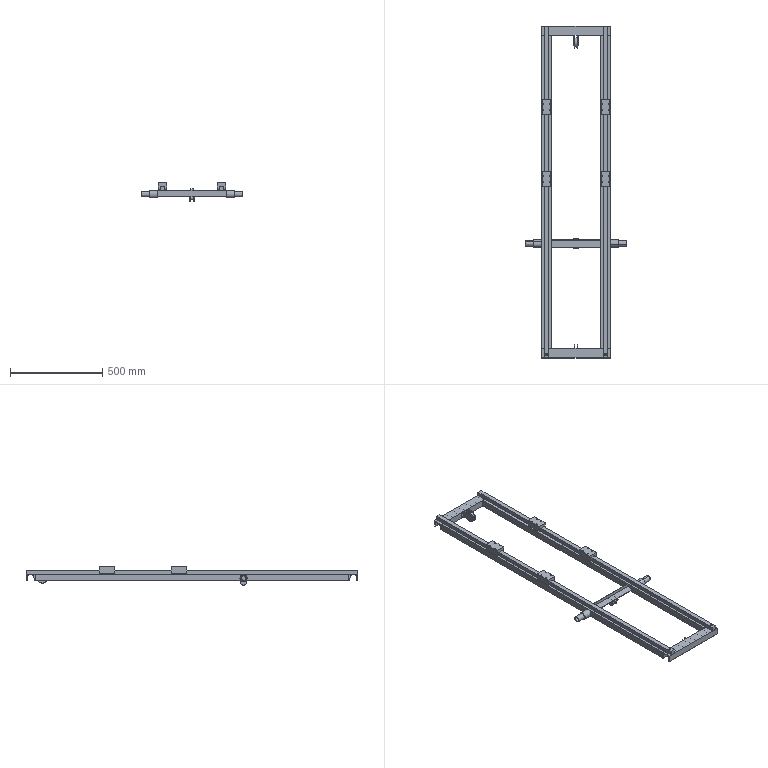Part | SolidWorks | 16 solids | 422 faces | box 550 x 1800 x 100 mm | volume 5250915 mm3 | cylinder 236 | plane 154 | cone 32 | commonest cylinder face diameters 6.5 x124 5 x40 6 x12 7 x12 4 x9 14 x8